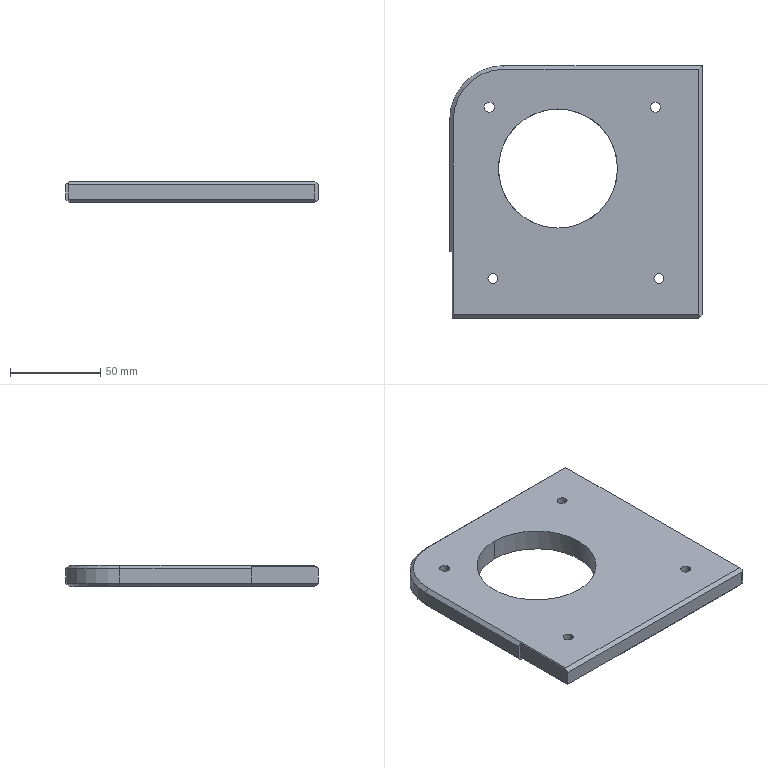Part | Creo | 1 solid | 43 faces | box 140 x 140 x 12 mm | volume 186778 mm3 | plane 22 | cylinder 19 | cone 2 | commonest cylinder face diameters 5.5 x8 9.5 x8 66 x2 60 x1
STEP:
#1=CARTESIAN_POINT('',(333.,-375.005,-1.));
#2=VERTEX_POINT('',#1);
#3=CARTESIAN_POINT('',(333.,-375.005,-9.));
#4=VERTEX_POINT('',#3);
#5=CARTESIAN_POINT('',(333.,-375.005,-1.));
#6=DIRECTION('',(0.,0.,-1.));
#7=VECTOR('',#6,8.);
#8=LINE('',#5,#7);
#9=EDGE_CURVE('',#2,#4,#8,.T.);
#10=ORIENTED_EDGE('',*,*,#9,.T.);
#11=CARTESIAN_POINT('',(196.5,-375.005,-9.));
#12=VERTEX_POINT('',#11);
#13=CARTESIAN_POINT('',(333.,-375.005,-9.));
#14=DIRECTION('',(-1.,0.,0.));
#15=VECTOR('',#14,136.5);
#16=LINE('',#13,#15);
#17=EDGE_CURVE('',#4,#12,#16,.T.);
#18=ORIENTED_EDGE('',*,*,#17,.T.);
#19=CARTESIAN_POINT('',(196.5,-375.005,-1.));
#20=VERTEX_POINT('',#19);
#21=CARTESIAN_POINT('',(196.5,-375.005,-1.));
#22=DIRECTION('',(0.,0.,-1.));
#23=VECTOR('',#22,8.);
#24=LINE('',#21,#23);
#25=EDGE_CURVE('',#20,#12,#24,.T.);
#26=ORIENTED_EDGE('',*,*,#25,.F.);
#27=CARTESIAN_POINT('',(196.5,-375.005,-1.));
#28=DIRECTION('',(1.,0.,0.));
#29=VECTOR('',#28,136.5);
#30=LINE('',#27,#29);
#31=EDGE_CURVE('',#20,#2,#30,.T.);
#32=ORIENTED_EDGE('',*,*,#31,.T.);
#33=EDGE_LOOP('',(#10,#18,#26,#32));
#34=FACE_OUTER_BOUND('',#33,.F.);
#35=CARTESIAN_POINT('',(-265.,-375.005,165.));
#36=DIRECTION('',(0.,-1.,0.));
#37=DIRECTION('',(0.,0.,-1.));
#38=AXIS2_PLACEMENT_3D('',#35,#36,#37);
#39=PLANE('',#38);
#40=ADVANCED_FACE('',(#34),#39,.T.);
#41=CARTESIAN_POINT('',(335.,-373.005,-9.));
#42=VERTEX_POINT('',#41);
#43=CARTESIAN_POINT('',(335.,-373.005,-1.));
#44=VERTEX_POINT('',#43);
#45=CARTESIAN_POINT('',(335.,-373.005,-9.));
#46=DIRECTION('',(0.,0.,1.));
#47=VECTOR('',#46,8.);
#48=LINE('',#45,#47);
#49=EDGE_CURVE('',#42,#44,#48,.T.);
#50=ORIENTED_EDGE('',*,*,#49,.F.);
#51=CARTESIAN_POINT('',(334.,-374.005,-10.));
#52=VERTEX_POINT('',#51);
#53=CARTESIAN_POINT('',(334.,-374.005,-10.));
#54=DIRECTION('',(0.5774,0.5774,0.5774));
#55=VECTOR('',#54,1.732);
#56=LINE('',#53,#55);
#57=EDGE_CURVE('',#52,#42,#56,.T.);
#58=ORIENTED_EDGE('',*,*,#57,.F.);
#59=CARTESIAN_POINT('',(333.,-375.005,-9.));
#60=DIRECTION('',(0.5774,0.5774,-0.5774));
#61=VECTOR('',#60,1.732);
#62=LINE('',#59,#61);
#63=EDGE_CURVE('',#4,#52,#62,.T.);
#64=ORIENTED_EDGE('',*,*,#63,.F.);
#65=ORIENTED_EDGE('',*,*,#9,.F.);
#66=CARTESIAN_POINT('',(334.,-374.005,0.));
#67=VERTEX_POINT('',#66);
#68=CARTESIAN_POINT('',(333.,-375.005,-1.));
#69=DIRECTION('',(0.5774,0.5774,0.5774));
#70=VECTOR('',#69,1.732);
#71=LINE('',#68,#70);
#72=EDGE_CURVE('',#2,#67,#71,.T.);
#73=ORIENTED_EDGE('',*,*,#72,.T.);
#74=CARTESIAN_POINT('',(334.,-374.005,0.));
#75=DIRECTION('',(0.5774,0.5774,-0.5774));
#76=VECTOR('',#75,1.732);
#77=LINE('',#74,#76);
#78=EDGE_CURVE('',#67,#44,#77,.T.);
#79=ORIENTED_EDGE('',*,*,#78,.T.);
#80=EDGE_LOOP('',(#50,#58,#64,#65,#73,#79));
#81=FACE_OUTER_BOUND('',#80,.F.);
#82=CARTESIAN_POINT('',(333.,-375.005,165.));
#83=DIRECTION('',(-0.7071,0.7071,0.));
#84=DIRECTION('',(0.,0.,1.));
#85=AXIS2_PLACEMENT_3D('',#82,#83,#84);
#86=PLANE('',#85);
#87=ADVANCED_FACE('',(#81),#86,.F.);
#88=CARTESIAN_POINT('',(335.,-235.005,-1.));
#89=VERTEX_POINT('',#88);
#90=CARTESIAN_POINT('',(335.,-235.005,-9.));
#91=VERTEX_POINT('',#90);
#92=CARTESIAN_POINT('',(335.,-235.005,-1.));
#93=DIRECTION('',(0.,0.,-1.));
#94=VECTOR('',#93,8.);
#95=LINE('',#92,#94);
#96=EDGE_CURVE('',#89,#91,#95,.T.);
#97=ORIENTED_EDGE('',*,*,#96,.T.);
#98=CARTESIAN_POINT('',(335.,-235.005,-9.));
#99=DIRECTION('',(0.,-1.,0.));
#100=VECTOR('',#99,138.);
#101=LINE('',#98,#100);
#102=EDGE_CURVE('',#91,#42,#101,.T.);
#103=ORIENTED_EDGE('',*,*,#102,.T.);
#104=ORIENTED_EDGE('',*,*,#49,.T.);
#105=CARTESIAN_POINT('',(335.,-373.005,-1.));
#106=DIRECTION('',(0.,1.,0.));
#107=VECTOR('',#106,138.);
#108=LINE('',#105,#107);
#109=EDGE_CURVE('',#44,#89,#108,.T.);
#110=ORIENTED_EDGE('',*,*,#109,.T.);
#111=EDGE_LOOP('',(#97,#103,#104,#110));
#112=FACE_OUTER_BOUND('',#111,.F.);
#113=CARTESIAN_POINT('',(335.,-50.005,5.));
#114=DIRECTION('',(1.,0.,0.));
#115=DIRECTION('',(0.,-1.,0.));
#116=AXIS2_PLACEMENT_3D('',#113,#114,#115);
#117=PLANE('',#116);
#118=ADVANCED_FACE('',(#112),#117,.T.);
#119=ORIENTED_EDGE('',*,*,#96,.F.);
#120=CARTESIAN_POINT('',(225.,-235.005,-1.));
#121=VERTEX_POINT('',#120);
#122=CARTESIAN_POINT('',(335.,-235.005,-1.));
#123=DIRECTION('',(-1.,0.,0.));
#124=VECTOR('',#123,110.);
#125=LINE('',#122,#124);
#126=EDGE_CURVE('',#89,#121,#125,.T.);
#127=ORIENTED_EDGE('',*,*,#126,.T.);
#128=CARTESIAN_POINT('',(225.,-235.005,-9.));
#129=VERTEX_POINT('',#128);
#130=CARTESIAN_POINT('',(225.,-235.005,-1.));
#131=DIRECTION('',(0.,0.,-1.));
#132=VECTOR('',#131,8.);
#133=LINE('',#130,#132);
#134=EDGE_CURVE('',#121,#129,#133,.T.);
#135=ORIENTED_EDGE('',*,*,#134,.T.);
#136=CARTESIAN_POINT('',(225.,-235.005,-9.));
#137=DIRECTION('',(1.,0.,0.));
#138=VECTOR('',#137,110.);
#139=LINE('',#136,#138);
#140=EDGE_CURVE('',#129,#91,#139,.T.);
#141=ORIENTED_EDGE('',*,*,#140,.T.);
#142=EDGE_LOOP('',(#119,#127,#135,#141));
#143=FACE_OUTER_BOUND('',#142,.F.);
#144=CARTESIAN_POINT('',(245.,-235.005,-10.));
#145=DIRECTION('',(0.,1.,0.));
#146=DIRECTION('',(0.,0.,1.));
#147=AXIS2_PLACEMENT_3D('',#144,#145,#146);
#148=PLANE('',#147);
#149=ADVANCED_FACE('',(#143),#148,.T.);
#150=CARTESIAN_POINT('',(225.,-237.005,1.));
#151=VERTEX_POINT('',#150);
#152=CARTESIAN_POINT('',(333.,-237.005,1.));
#153=VERTEX_POINT('',#152);
#154=CARTESIAN_POINT('',(225.,-237.005,1.));
#155=DIRECTION('',(1.,0.,0.));
#156=VECTOR('',#155,108.);
#157=LINE('',#154,#156);
#158=EDGE_CURVE('',#151,#153,#157,.T.);
#159=ORIENTED_EDGE('',*,*,#158,.F.);
#160=CARTESIAN_POINT('',(225.,-237.005,1.));
#161=DIRECTION('',(0.,0.7071,-0.7071));
#162=VECTOR('',#161,2.828);
#163=LINE('',#160,#162);
#164=EDGE_CURVE('',#151,#121,#163,.T.);
#165=ORIENTED_EDGE('',*,*,#164,.T.);
#166=ORIENTED_EDGE('',*,*,#126,.F.);
#167=CARTESIAN_POINT('',(335.,-235.005,-1.));
#168=DIRECTION('',(-0.5774,-0.5774,0.5774));
#169=VECTOR('',#168,3.464);
#170=LINE('',#167,#169);
#171=EDGE_CURVE('',#89,#153,#170,.T.);
#172=ORIENTED_EDGE('',*,*,#171,.T.);
#173=EDGE_LOOP('',(#159,#165,#166,#172));
#174=FACE_OUTER_BOUND('',#173,.F.);
#175=CARTESIAN_POINT('',(245.,-235.005,-1.));
#176=DIRECTION('',(0.,-0.7071,-0.7071));
#177=DIRECTION('',(1.,0.,0.));
#178=AXIS2_PLACEMENT_3D('',#175,#176,#177);
#179=PLANE('',#178);
#180=ADVANCED_FACE('',(#174),#179,.F.);
#181=CARTESIAN_POINT('',(333.,-373.005,1.));
#182=VERTEX_POINT('',#181);
#183=CARTESIAN_POINT('',(197.,-373.005,1.));
#184=VERTEX_POINT('',#183);
#185=CARTESIAN_POINT('',(333.,-373.005,1.));
#186=DIRECTION('',(-1.,0.,0.));
#187=VECTOR('',#186,136.);
#188=LINE('',#185,#187);
#189=EDGE_CURVE('',#182,#184,#188,.T.);
#190=ORIENTED_EDGE('',*,*,#189,.T.);
#191=CARTESIAN_POINT('',(197.,-265.005,1.));
#192=VERTEX_POINT('',#191);
#193=CARTESIAN_POINT('',(197.,-373.005,1.));
#194=DIRECTION('',(0.,1.,0.));
#195=VECTOR('',#194,108.);
#196=LINE('',#193,#195);
#197=EDGE_CURVE('',#184,#192,#196,.T.);
#198=ORIENTED_EDGE('',*,*,#197,.T.);
#199=CARTESIAN_POINT('',(225.,-265.005,1.));
#200=DIRECTION('',(0.,0.,1.));
#201=DIRECTION('',(0.,1.,0.));
#202=AXIS2_PLACEMENT_3D('',#199,#200,#201);
#203=CIRCLE('',#202,28.);
#204=EDGE_CURVE('',#151,#192,#203,.T.);
#205=ORIENTED_EDGE('',*,*,#204,.F.);
#206=ORIENTED_EDGE('',*,*,#158,.T.);
#207=CARTESIAN_POINT('',(333.,-237.005,1.));
#208=DIRECTION('',(0.,-1.,0.));
#209=VECTOR('',#208,136.);
#210=LINE('',#207,#209);
#211=EDGE_CURVE('',#153,#182,#210,.T.);
#212=ORIENTED_EDGE('',*,*,#211,.T.);
#213=EDGE_LOOP('',(#190,#198,#205,#206,#212));
#214=FACE_OUTER_BOUND('',#213,.F.);
#215=CARTESIAN_POINT('',(306.25,-258.009,1.));
#216=VERTEX_POINT('',#215);
#217=CARTESIAN_POINT('',(311.75,-258.009,1.));
#218=VERTEX_POINT('',#217);
#219=CARTESIAN_POINT('',(309.,-258.009,1.));
#220=DIRECTION('',(0.,0.,-1.));
#221=DIRECTION('',(-1.,0.,0.));
#222=AXIS2_PLACEMENT_3D('',#219,#220,#221);
#223=CIRCLE('',#222,2.75);
#224=EDGE_CURVE('',#216,#218,#223,.T.);
#225=ORIENTED_EDGE('',*,*,#224,.F.);
#226=CARTESIAN_POINT('',(309.,-258.009,1.));
#227=DIRECTION('',(0.,0.,-1.));
#228=DIRECTION('',(1.,0.,0.));
#229=AXIS2_PLACEMENT_3D('',#226,#227,#228);
#230=CIRCLE('',#229,2.75);
#231=EDGE_CURVE('',#218,#216,#230,.T.);
#232=ORIENTED_EDGE('',*,*,#231,.F.);
#233=EDGE_LOOP('',(#225,#232));
#234=FACE_BOUND('',#233,.F.);
#235=CARTESIAN_POINT('',(216.199,-353.009,1.));
#236=VERTEX_POINT('',#235);
#237=CARTESIAN_POINT('',(221.699,-353.009,1.));
#238=VERTEX_POINT('',#237);
#239=CARTESIAN_POINT('',(218.949,-353.009,1.));
#240=DIRECTION('',(0.,0.,-1.));
#241=DIRECTION('',(-1.,0.,0.));
#242=AXIS2_PLACEMENT_3D('',#239,#240,#241);
#243=CIRCLE('',#242,2.75);
#244=EDGE_CURVE('',#236,#238,#243,.T.);
#245=ORIENTED_EDGE('',*,*,#244,.F.);
#246=CARTESIAN_POINT('',(218.949,-353.009,1.));
#247=DIRECTION('',(0.,0.,-1.));
#248=DIRECTION('',(1.,0.,0.));
#249=AXIS2_PLACEMENT_3D('',#246,#247,#248);
#250=CIRCLE('',#249,2.75);
#251=EDGE_CURVE('',#238,#236,#250,.T.);
#252=ORIENTED_EDGE('',*,*,#251,.F.);
#253=EDGE_LOOP('',(#245,#252));
#254=FACE_BOUND('',#253,.F.);
#255=CARTESIAN_POINT('',(288.,-292.005,1.));
#256=VERTEX_POINT('',#255);
#257=CARTESIAN_POINT('',(255.,-325.005,1.));
#258=VERTEX_POINT('',#257);
#259=CARTESIAN_POINT('',(255.,-292.005,1.));
#260=DIRECTION('',(0.,0.,-1.));
#261=DIRECTION('',(1.,0.,0.));
#262=AXIS2_PLACEMENT_3D('',#259,#260,#261);
#263=CIRCLE('',#262,33.);
#264=EDGE_CURVE('',#256,#258,#263,.T.);
#265=ORIENTED_EDGE('',*,*,#264,.F.);
#266=CARTESIAN_POINT('',(255.,-259.005,1.));
#267=VERTEX_POINT('',#266);
#268=CARTESIAN_POINT('',(255.,-292.005,1.));
#269=DIRECTION('',(0.,0.,-1.));
#270=DIRECTION('',(0.,1.,0.));
#271=AXIS2_PLACEMENT_3D('',#268,#269,#270);
#272=CIRCLE('',#271,33.);
#273=EDGE_CURVE('',#267,#256,#272,.T.);
#274=ORIENTED_EDGE('',*,*,#273,.F.);
#275=CARTESIAN_POINT('',(255.,-292.005,1.));
#276=DIRECTION('',(0.,0.,-1.));
#277=DIRECTION('',(0.,-1.,0.));
#278=AXIS2_PLACEMENT_3D('',#275,#276,#277);
#279=CIRCLE('',#278,33.);
#280=EDGE_CURVE('',#258,#267,#279,.T.);
#281=ORIENTED_EDGE('',*,*,#280,.F.);
#282=EDGE_LOOP('',(#265,#274,#281));
#283=FACE_BOUND('',#282,.F.);
#284=CARTESIAN_POINT('',(214.25,-258.009,1.));
#285=VERTEX_POINT('',#284);
#286=CARTESIAN_POINT('',(219.75,-258.009,1.));
#287=VERTEX_POINT('',#286);
#288=CARTESIAN_POINT('',(217.,-258.009,1.));
#289=DIRECTION('',(0.,0.,-1.));
#290=DIRECTION('',(-1.,0.,0.));
#291=AXIS2_PLACEMENT_3D('',#288,#289,#290);
#292=CIRCLE('',#291,2.75);
#293=EDGE_CURVE('',#285,#287,#292,.T.);
#294=ORIENTED_EDGE('',*,*,#293,.F.);
#295=CARTESIAN_POINT('',(217.,-258.009,1.));
#296=DIRECTION('',(0.,0.,-1.));
#297=DIRECTION('',(1.,0.,0.));
#298=AXIS2_PLACEMENT_3D('',#295,#296,#297);
#299=CIRCLE('',#298,2.75);
#300=EDGE_CURVE('',#287,#285,#299,.T.);
#301=ORIENTED_EDGE('',*,*,#300,.F.);
#302=EDGE_LOOP('',(#294,#301));
#303=FACE_BOUND('',#302,.F.);
#304=CARTESIAN_POINT('',(308.199,-353.009,1.));
#305=VERTEX_POINT('',#304);
#306=CARTESIAN_POINT('',(313.699,-353.009,1.));
#307=VERTEX_POINT('',#306);
#308=CARTESIAN_POINT('',(310.949,-353.009,1.));
#309=DIRECTION('',(0.,0.,-1.));
#310=DIRECTION('',(-1.,0.,0.));
#311=AXIS2_PLACEMENT_3D('',#308,#309,#310);
#312=CIRCLE('',#311,2.75);
#313=EDGE_CURVE('',#305,#307,#312,.T.);
#314=ORIENTED_EDGE('',*,*,#313,.F.);
#315=CARTESIAN_POINT('',(310.949,-353.009,1.));
#316=DIRECTION('',(0.,0.,-1.));
#317=DIRECTION('',(1.,0.,0.));
#318=AXIS2_PLACEMENT_3D('',#315,#316,#317);
#319=CIRCLE('',#318,2.75);
#320=EDGE_CURVE('',#307,#305,#319,.T.);
#321=ORIENTED_EDGE('',*,*,#320,.F.);
#322=EDGE_LOOP('',(#314,#321));
#323=FACE_BOUND('',#322,.F.);
#324=CARTESIAN_POINT('',(245.,-302.505,1.));
#325=DIRECTION('',(0.,0.,1.));
#326=DIRECTION('',(1.,0.,0.));
#327=AXIS2_PLACEMENT_3D('',#324,#325,#326);
#328=PLANE('',#327);
#329=ADVANCED_FACE('',(#214,#234,#254,#283,#303,#323),#328,.T.);
#330=ORIENTED_EDGE('',*,*,#72,.F.);
#331=ORIENTED_EDGE('',*,*,#31,.F.);
#332=CARTESIAN_POINT('',(196.5,-373.505,0.5));
#333=VERTEX_POINT('',#332);
#334=CARTESIAN_POINT('',(196.5,-375.005,-1.));
#335=DIRECTION('',(0.,0.7071,0.7071));
#336=VECTOR('',#335,2.121);
#337=LINE('',#334,#336);
#338=EDGE_CURVE('',#20,#333,#337,.T.);
#339=ORIENTED_EDGE('',*,*,#338,.T.);
#340=CARTESIAN_POINT('',(197.,-373.005,1.));
#341=DIRECTION('',(-0.5774,-0.5774,-0.5774));
#342=VECTOR('',#341,0.866);
#343=LINE('',#340,#342);
#344=EDGE_CURVE('',#184,#333,#343,.T.);
#345=ORIENTED_EDGE('',*,*,#344,.F.);
#346=ORIENTED_EDGE('',*,*,#189,.F.);
#347=CARTESIAN_POINT('',(333.,-373.005,1.));
#348=DIRECTION('',(0.5774,-0.5774,-0.5774));
#349=VECTOR('',#348,1.732);
#350=LINE('',#347,#349);
#351=EDGE_CURVE('',#182,#67,#350,.T.);
#352=ORIENTED_EDGE('',*,*,#351,.T.);
#353=EDGE_LOOP('',(#330,#331,#339,#345,#346,#352));
#354=FACE_OUTER_BOUND('',#353,.F.);
#355=CARTESIAN_POINT('',(245.,-373.005,1.));
#356=DIRECTION('',(0.,0.7071,-0.7071));
#357=DIRECTION('',(1.,0.,0.));
#358=AXIS2_PLACEMENT_3D('',#355,#356,#357);
#359=PLANE('',#358);
#360=ADVANCED_FACE('',(#354),#359,.F.);
#361=ORIENTED_EDGE('',*,*,#25,.T.);
#362=CARTESIAN_POINT('',(196.5,-338.005,-9.));
#363=VERTEX_POINT('',#362);
#364=CARTESIAN_POINT('',(196.5,-375.005,-9.));
#365=DIRECTION('',(0.,1.,0.));
#366=VECTOR('',#365,37.);
#367=LINE('',#364,#366);
#368=EDGE_CURVE('',#12,#363,#367,.T.);
#369=ORIENTED_EDGE('',*,*,#368,.T.);
#370=CARTESIAN_POINT('',(196.5,-338.005,0.5));
#371=VERTEX_POINT('',#370);
#372=CARTESIAN_POINT('',(196.5,-338.005,-9.));
#373=DIRECTION('',(0.,0.,1.));
#374=VECTOR('',#373,9.5);
#375=LINE('',#372,#374);
#376=EDGE_CURVE('',#363,#371,#375,.T.);
#377=ORIENTED_EDGE('',*,*,#376,.T.);
#378=CARTESIAN_POINT('',(196.5,-338.005,0.5));
#379=DIRECTION('',(0.,-1.,0.));
#380=VECTOR('',#379,35.5);
#381=LINE('',#378,#380);
#382=EDGE_CURVE('',#371,#333,#381,.T.);
#383=ORIENTED_EDGE('',*,*,#382,.T.);
#384=ORIENTED_EDGE('',*,*,#338,.F.);
#385=EDGE_LOOP('',(#361,#369,#377,#383,#384));
#386=FACE_OUTER_BOUND('',#385,.F.);
#387=CARTESIAN_POINT('',(196.5,-394.005,-194.076));
#388=DIRECTION('',(1.,0.,0.));
#389=DIRECTION('',(0.,0.,1.));
#390=AXIS2_PLACEMENT_3D('',#387,#388,#389);
#391=PLANE('',#390);
#392=ADVANCED_FACE('',(#386),#391,.F.);
#393=CARTESIAN_POINT('',(198.5,-338.005,-11.));
#394=VERTEX_POINT('',#393);
#395=CARTESIAN_POINT('',(198.5,-338.005,-11.));
#396=DIRECTION('',(-0.7071,0.,0.7071));
#397=VECTOR('',#396,2.828);
#398=LINE('',#395,#397);
#399=EDGE_CURVE('',#394,#363,#398,.T.);
#400=ORIENTED_EDGE('',*,*,#399,.T.);
#401=ORIENTED_EDGE('',*,*,#368,.F.);
#402=CARTESIAN_POINT('',(198.5,-373.005,-11.));
#403=VERTEX_POINT('',#402);
#404=CARTESIAN_POINT('',(198.5,-373.005,-11.));
#405=DIRECTION('',(-0.5774,-0.5774,0.5774));
#406=VECTOR('',#405,3.464);
#407=LINE('',#404,#406);
#408=EDGE_CURVE('',#403,#12,#407,.T.);
#409=ORIENTED_EDGE('',*,*,#408,.F.);
#410=CARTESIAN_POINT('',(198.5,-338.005,-11.));
#411=DIRECTION('',(0.,-1.,0.));
#412=VECTOR('',#411,35.);
#413=LINE('',#410,#412);
#414=EDGE_CURVE('',#394,#403,#413,.T.);
#415=ORIENTED_EDGE('',*,*,#414,.F.);
#416=EDGE_LOOP('',(#400,#401,#409,#415));
#417=FACE_OUTER_BOUND('',#416,.F.);
#418=CARTESIAN_POINT('',(196.5,-394.005,-9.));
#419=DIRECTION('',(-0.7071,0.,-0.7071));
#420=DIRECTION('',(0.,1.,0.));
#421=AXIS2_PLACEMENT_3D('',#418,#419,#420);
#422=PLANE('',#421);
#423=ADVANCED_FACE('',(#417),#422,.T.);
#424=CARTESIAN_POINT('',(195.,-338.005,-9.));
#425=VERTEX_POINT('',#424);
#426=CARTESIAN_POINT('',(195.,-338.005,-1.));
#427=VERTEX_POINT('',#426);
#428=CARTESIAN_POINT('',(195.,-338.005,-9.));
#429=DIRECTION('',(0.,0.,1.));
#430=VECTOR('',#429,8.);
#431=LINE('',#428,#430);
#432=EDGE_CURVE('',#425,#427,#431,.T.);
#433=ORIENTED_EDGE('',*,*,#432,.T.);
#434=CARTESIAN_POINT('',(196.5,-338.005,0.5));
#435=DIRECTION('',(-0.7071,0.,-0.7071));
#436=VECTOR('',#435,2.121);
#437=LINE('',#434,#436);
#438=EDGE_CURVE('',#371,#427,#437,.T.);
#439=ORIENTED_EDGE('',*,*,#438,.F.);
#440=ORIENTED_EDGE('',*,*,#376,.F.);
#441=ORIENTED_EDGE('',*,*,#399,.F.);
#442=CARTESIAN_POINT('',(197.,-338.005,-11.));
#443=VERTEX_POINT('',#442);
#444=CARTESIAN_POINT('',(198.5,-338.005,-11.));
#445=DIRECTION('',(-1.,0.,0.));
#446=VECTOR('',#445,1.5);
#447=LINE('',#444,#446);
#448=EDGE_CURVE('',#394,#443,#447,.T.);
#449=ORIENTED_EDGE('',*,*,#448,.T.);
#450=CARTESIAN_POINT('',(195.,-338.005,-9.));
#451=DIRECTION('',(0.7071,0.,-0.7071));
#452=VECTOR('',#451,2.828);
#453=LINE('',#450,#452);
#454=EDGE_CURVE('',#425,#443,#453,.T.);
#455=ORIENTED_EDGE('',*,*,#454,.F.);
#456=EDGE_LOOP('',(#433,#439,#440,#441,#449,#455));
#457=FACE_OUTER_BOUND('',#456,.F.);
#458=CARTESIAN_POINT('',(175.,-338.005,-20.));
#459=DIRECTION('',(0.,-1.,0.));
#460=DIRECTION('',(1.,0.,0.));
#461=AXIS2_PLACEMENT_3D('',#458,#459,#460);
#462=PLANE('',#461);
#463=ADVANCED_FACE('',(#457),#462,.T.);
#464=CARTESIAN_POINT('',(195.,-265.005,-9.));
#465=VERTEX_POINT('',#464);
#466=CARTESIAN_POINT('',(195.,-265.005,-1.));
#467=VERTEX_POINT('',#466);
#468=CARTESIAN_POINT('',(195.,-265.005,-9.));
#469=DIRECTION('',(0.,0.,1.));
#470=VECTOR('',#469,8.);
#471=LINE('',#468,#470);
#472=EDGE_CURVE('',#465,#467,#471,.T.);
#473=ORIENTED_EDGE('',*,*,#472,.T.);
#474=CARTESIAN_POINT('',(195.,-265.005,-1.));
#475=DIRECTION('',(0.,-1.,0.));
#476=VECTOR('',#475,73.);
#477=LINE('',#474,#476);
#478=EDGE_CURVE('',#467,#427,#477,.T.);
#479=ORIENTED_EDGE('',*,*,#478,.T.);
#480=ORIENTED_EDGE('',*,*,#432,.F.);
#481=CARTESIAN_POINT('',(195.,-338.005,-9.));
#482=DIRECTION('',(0.,1.,0.));
#483=VECTOR('',#482,73.);
#484=LINE('',#481,#483);
#485=EDGE_CURVE('',#425,#465,#484,.T.);
#486=ORIENTED_EDGE('',*,*,#485,.T.);
#487=EDGE_LOOP('',(#473,#479,#480,#486));
#488=FACE_OUTER_BOUND('',#487,.F.);
#489=CARTESIAN_POINT('',(195.,-0.004699,1.));
#490=DIRECTION('',(1.,0.,0.));
#491=DIRECTION('',(0.,-1.,0.));
#492=AXIS2_PLACEMENT_3D('',#489,#490,#491);
#493=PLANE('',#492);
#494=ADVANCED_FACE('',(#488),#493,.F.);
#495=ORIENTED_EDGE('',*,*,#134,.F.);
#496=CARTESIAN_POINT('',(225.,-265.005,-1.));
#497=DIRECTION('',(0.,0.,1.));
#498=DIRECTION('',(0.,1.,0.));
#499=AXIS2_PLACEMENT_3D('',#496,#497,#498);
#500=CIRCLE('',#499,30.);
#501=EDGE_CURVE('',#121,#467,#500,.T.);
#502=ORIENTED_EDGE('',*,*,#501,.T.);
#503=ORIENTED_EDGE('',*,*,#472,.F.);
#504=CARTESIAN_POINT('',(225.,-265.005,-9.));
#505=DIRECTION('',(0.,0.,-1.));
#506=DIRECTION('',(-1.,0.,0.));
#507=AXIS2_PLACEMENT_3D('',#504,#505,#506);
#508=CIRCLE('',#507,30.);
#509=EDGE_CURVE('',#465,#129,#508,.T.);
#510=ORIENTED_EDGE('',*,*,#509,.T.);
#511=EDGE_LOOP('',(#495,#502,#503,#510));
#512=FACE_OUTER_BOUND('',#511,.F.);
#513=CARTESIAN_POINT('',(225.,-265.005,-10.));
#514=DIRECTION('',(0.,0.,-1.));
#515=DIRECTION('',(-1.,0.,0.));
#516=AXIS2_PLACEMENT_3D('',#513,#514,#515);
#517=CYLINDRICAL_SURFACE('',#516,30.);
#518=ADVANCED_FACE('',(#512),#517,.T.);
#519=ORIENTED_EDGE('',*,*,#164,.F.);
#520=ORIENTED_EDGE('',*,*,#204,.T.);
#521=CARTESIAN_POINT('',(195.,-265.005,-1.));
#522=DIRECTION('',(0.7071,0.,0.7071));
#523=VECTOR('',#522,2.828);
#524=LINE('',#521,#523);
#525=EDGE_CURVE('',#467,#192,#524,.T.);
#526=ORIENTED_EDGE('',*,*,#525,.F.);
#527=ORIENTED_EDGE('',*,*,#501,.F.);
#528=EDGE_LOOP('',(#519,#520,#526,#527));
#529=FACE_OUTER_BOUND('',#528,.F.);
#530=CARTESIAN_POINT('',(225.,-265.005,0.));
#531=DIRECTION('',(0.,0.,-1.));
#532=DIRECTION('',(-1.,0.,0.));
#533=AXIS2_PLACEMENT_3D('',#530,#531,#532);
#534=CONICAL_SURFACE('',#533,29.,45.);
#535=ADVANCED_FACE('',(#529),#534,.T.);
#536=ORIENTED_EDGE('',*,*,#382,.F.);
#537=ORIENTED_EDGE('',*,*,#438,.T.);
#538=ORIENTED_EDGE('',*,*,#478,.F.);
#539=ORIENTED_EDGE('',*,*,#525,.T.);
#540=ORIENTED_EDGE('',*,*,#197,.F.);
#541=ORIENTED_EDGE('',*,*,#344,.T.);
#542=EDGE_LOOP('',(#536,#537,#538,#539,#540,#541));
#543=FACE_OUTER_BOUND('',#542,.F.);
#544=CARTESIAN_POINT('',(195.,-0.004699,-1.));
#545=DIRECTION('',(-0.7071,0.,0.7071));
#546=DIRECTION('',(0.,-1.,0.));
#547=AXIS2_PLACEMENT_3D('',#544,#545,#546);
#548=PLANE('',#547);
#549=ADVANCED_FACE('',(#543),#548,.T.);
#550=CARTESIAN_POINT('',(197.,-265.005,-11.));
#551=VERTEX_POINT('',#550);
#552=CARTESIAN_POINT('',(197.,-265.005,-11.));
#553=DIRECTION('',(-0.7071,0.,0.7071));
#554=VECTOR('',#553,2.828);
#555=LINE('',#552,#554);
#556=EDGE_CURVE('',#551,#465,#555,.T.);
#557=ORIENTED_EDGE('',*,*,#556,.F.);
#558=CARTESIAN_POINT('',(225.,-237.005,-11.));
#559=VERTEX_POINT('',#558);
#560=CARTESIAN_POINT('',(225.,-265.005,-11.));
#561=DIRECTION('',(0.,0.,-1.));
#562=DIRECTION('',(-1.,0.,0.));
#563=AXIS2_PLACEMENT_3D('',#560,#561,#562);
#564=CIRCLE('',#563,28.);
#565=EDGE_CURVE('',#551,#559,#564,.T.);
#566=ORIENTED_EDGE('',*,*,#565,.T.);
#567=CARTESIAN_POINT('',(225.,-235.005,-9.));
#568=DIRECTION('',(0.,-0.7071,-0.7071));
#569=VECTOR('',#568,2.828);
#570=LINE('',#567,#569);
#571=EDGE_CURVE('',#129,#559,#570,.T.);
#572=ORIENTED_EDGE('',*,*,#571,.F.);
#573=ORIENTED_EDGE('',*,*,#509,.F.);
#574=EDGE_LOOP('',(#557,#566,#572,#573));
#575=FACE_OUTER_BOUND('',#574,.F.);
#576=CARTESIAN_POINT('',(225.,-265.005,-10.));
#577=DIRECTION('',(0.,0.,1.));
#578=DIRECTION('',(1.,0.,0.));
#579=AXIS2_PLACEMENT_3D('',#576,#577,#578);
#580=CONICAL_SURFACE('',#579,29.,45.);
#581=ADVANCED_FACE('',(#575),#580,.T.);
#582=ORIENTED_EDGE('',*,*,#454,.T.);
#583=CARTESIAN_POINT('',(197.,-265.005,-11.));
#584=DIRECTION('',(0.,-1.,0.));
#585=VECTOR('',#584,73.);
#586=LINE('',#583,#585);
#587=EDGE_CURVE('',#551,#443,#586,.T.);
#588=ORIENTED_EDGE('',*,*,#587,.F.);
#589=ORIENTED_EDGE('',*,*,#556,.T.);
#590=ORIENTED_EDGE('',*,*,#485,.F.);
#591=EDGE_LOOP('',(#582,#588,#589,#590));
#592=FACE_OUTER_BOUND('',#591,.F.);
#593=CARTESIAN_POINT('',(195.,-0.004699,-9.));
#594=DIRECTION('',(-0.7071,0.,-0.7071));
#595=DIRECTION('',(0.,1.,0.));
#596=AXIS2_PLACEMENT_3D('',#593,#594,#595);
#597=PLANE('',#596);
#598=ADVANCED_FACE('',(#592),#597,.T.);
#599=ORIENTED_EDGE('',*,*,#565,.F.);
#600=ORIENTED_EDGE('',*,*,#587,.T.);
#601=ORIENTED_EDGE('',*,*,#448,.F.);
#602=ORIENTED_EDGE('',*,*,#414,.T.);
#603=CARTESIAN_POINT('',(333.,-373.005,-11.));
#604=VERTEX_POINT('',#603);
#605=CARTESIAN_POINT('',(198.5,-373.005,-11.));
#606=DIRECTION('',(1.,0.,0.));
#607=VECTOR('',#606,134.5);
#608=LINE('',#605,#607);
#609=EDGE_CURVE('',#403,#604,#608,.T.);
#610=ORIENTED_EDGE('',*,*,#609,.T.);
#611=CARTESIAN_POINT('',(333.,-237.005,-11.));
#612=VERTEX_POINT('',#611);
#613=CARTESIAN_POINT('',(333.,-373.005,-11.));
#614=DIRECTION('',(0.,1.,0.));
#615=VECTOR('',#614,136.);
#616=LINE('',#613,#615);
#617=EDGE_CURVE('',#604,#612,#616,.T.);
#618=ORIENTED_EDGE('',*,*,#617,.T.);
#619=CARTESIAN_POINT('',(333.,-237.005,-11.));
#620=DIRECTION('',(-1.,0.,0.));
#621=VECTOR('',#620,108.);
#622=LINE('',#619,#621);
#623=EDGE_CURVE('',#612,#559,#622,.T.);
#624=ORIENTED_EDGE('',*,*,#623,.T.);
#625=EDGE_LOOP('',(#599,#600,#601,#602,#610,#618,#624));
#626=FACE_OUTER_BOUND('',#625,.F.);
#627=CARTESIAN_POINT('',(214.199,-353.009,-11.));
#628=VERTEX_POINT('',#627);
#629=CARTESIAN_POINT('',(223.699,-353.009,-11.));
#630=VERTEX_POINT('',#629);
#631=CARTESIAN_POINT('',(218.949,-353.009,-11.));
#632=DIRECTION('',(0.,0.,1.));
#633=DIRECTION('',(-1.,0.,0.));
#634=AXIS2_PLACEMENT_3D('',#631,#632,#633);
#635=CIRCLE('',#634,4.75);
#636=EDGE_CURVE('',#628,#630,#635,.T.);
#637=ORIENTED_EDGE('',*,*,#636,.F.);
#638=CARTESIAN_POINT('',(218.949,-353.009,-11.));
#639=DIRECTION('',(0.,0.,1.));
#640=DIRECTION('',(1.,0.,0.));
#641=AXIS2_PLACEMENT_3D('',#638,#639,#640);
#642=CIRCLE('',#641,4.75);
#643=EDGE_CURVE('',#630,#628,#642,.T.);
#644=ORIENTED_EDGE('',*,*,#643,.F.);
#645=EDGE_LOOP('',(#637,#644));
#646=FACE_BOUND('',#645,.F.);
#647=CARTESIAN_POINT('',(306.199,-353.009,-11.));
#648=VERTEX_POINT('',#647);
#649=CARTESIAN_POINT('',(315.699,-353.009,-11.));
#650=VERTEX_POINT('',#649);
#651=CARTESIAN_POINT('',(310.949,-353.009,-11.));
#652=DIRECTION('',(0.,0.,1.));
#653=DIRECTION('',(-1.,0.,0.));
#654=AXIS2_PLACEMENT_3D('',#651,#652,#653);
#655=CIRCLE('',#654,4.75);
#656=EDGE_CURVE('',#648,#650,#655,.T.);
#657=ORIENTED_EDGE('',*,*,#656,.F.);
#658=CARTESIAN_POINT('',(310.949,-353.009,-11.));
#659=DIRECTION('',(0.,0.,1.));
#660=DIRECTION('',(1.,0.,0.));
#661=AXIS2_PLACEMENT_3D('',#658,#659,#660);
#662=CIRCLE('',#661,4.75);
#663=EDGE_CURVE('',#650,#648,#662,.T.);
#664=ORIENTED_EDGE('',*,*,#663,.F.);
#665=EDGE_LOOP('',(#657,#664));
#666=FACE_BOUND('',#665,.F.);
#667=CARTESIAN_POINT('',(304.25,-258.009,-11.));
#668=VERTEX_POINT('',#667);
#669=CARTESIAN_POINT('',(313.75,-258.009,-11.));
#670=VERTEX_POINT('',#669);
#671=CARTESIAN_POINT('',(309.,-258.009,-11.));
#672=DIRECTION('',(0.,0.,1.));
#673=DIRECTION('',(-1.,0.,0.));
#674=AXIS2_PLACEMENT_3D('',#671,#672,#673);
#675=CIRCLE('',#674,4.75);
#676=EDGE_CURVE('',#668,#670,#675,.T.);
#677=ORIENTED_EDGE('',*,*,#676,.F.);
#678=CARTESIAN_POINT('',(309.,-258.009,-11.));
#679=DIRECTION('',(0.,0.,1.));
#680=DIRECTION('',(1.,0.,0.));
#681=AXIS2_PLACEMENT_3D('',#678,#679,#680);
#682=CIRCLE('',#681,4.75);
#683=EDGE_CURVE('',#670,#668,#682,.T.);
#684=ORIENTED_EDGE('',*,*,#683,.F.);
#685=EDGE_LOOP('',(#677,#684));
#686=FACE_BOUND('',#685,.F.);
#687=CARTESIAN_POINT('',(212.25,-258.009,-11.));
#688=VERTEX_POINT('',#687);
#689=CARTESIAN_POINT('',(221.75,-258.009,-11.));
#690=VERTEX_POINT('',#689);
#691=CARTESIAN_POINT('',(217.,-258.009,-11.));
#692=DIRECTION('',(0.,0.,1.));
#693=DIRECTION('',(-1.,0.,0.));
#694=AXIS2_PLACEMENT_3D('',#691,#692,#693);
#695=CIRCLE('',#694,4.75);
#696=EDGE_CURVE('',#688,#690,#695,.T.);
#697=ORIENTED_EDGE('',*,*,#696,.F.);
#698=CARTESIAN_POINT('',(217.,-258.009,-11.));
#699=DIRECTION('',(0.,0.,1.));
#700=DIRECTION('',(1.,0.,0.));
#701=AXIS2_PLACEMENT_3D('',#698,#699,#700);
#702=CIRCLE('',#701,4.75);
#703=EDGE_CURVE('',#690,#688,#702,.T.);
#704=ORIENTED_EDGE('',*,*,#703,.F.);
#705=EDGE_LOOP('',(#697,#704));
#706=FACE_BOUND('',#705,.F.);
#707=CARTESIAN_POINT('',(222.,-292.005,-11.));
#708=VERTEX_POINT('',#707);
#709=CARTESIAN_POINT('',(255.,-325.005,-11.));
#710=VERTEX_POINT('',#709);
#711=CARTESIAN_POINT('',(255.,-292.005,-11.));
#712=DIRECTION('',(0.,0.,1.));
#713=DIRECTION('',(-1.,0.,0.));
#714=AXIS2_PLACEMENT_3D('',#711,#712,#713);
#715=CIRCLE('',#714,33.);
#716=EDGE_CURVE('',#708,#710,#715,.T.);
#717=ORIENTED_EDGE('',*,*,#716,.F.);
#718=CARTESIAN_POINT('',(255.,-259.005,-11.));
#719=VERTEX_POINT('',#718);
#720=CARTESIAN_POINT('',(255.,-292.005,-11.));
#721=DIRECTION('',(0.,0.,1.));
#722=DIRECTION('',(0.,1.,0.));
#723=AXIS2_PLACEMENT_3D('',#720,#721,#722);
#724=CIRCLE('',#723,33.);
#725=EDGE_CURVE('',#719,#708,#724,.T.);
#726=ORIENTED_EDGE('',*,*,#725,.F.);
#727=CARTESIAN_POINT('',(255.,-292.005,-11.));
#728=DIRECTION('',(0.,0.,1.));
#729=DIRECTION('',(0.,-1.,0.));
#730=AXIS2_PLACEMENT_3D('',#727,#728,#729);
#731=CIRCLE('',#730,33.);
#732=EDGE_CURVE('',#710,#719,#731,.T.);
#733=ORIENTED_EDGE('',*,*,#732,.F.);
#734=EDGE_LOOP('',(#717,#726,#733));
#735=FACE_BOUND('',#734,.F.);
#736=CARTESIAN_POINT('',(245.,-302.505,-11.));
#737=DIRECTION('',(0.,0.,-1.));
#738=DIRECTION('',(-1.,0.,0.));
#739=AXIS2_PLACEMENT_3D('',#736,#737,#738);
#740=PLANE('',#739);
#741=ADVANCED_FACE('',(#626,#646,#666,#686,#706,#735),#740,.T.);
#742=CARTESIAN_POINT('',(333.,-373.005,-11.));
#743=DIRECTION('',(0.5774,-0.5774,0.5774));
#744=VECTOR('',#743,1.732);
#745=LINE('',#742,#744);
#746=EDGE_CURVE('',#604,#52,#745,.T.);
#747=ORIENTED_EDGE('',*,*,#746,.F.);
#748=ORIENTED_EDGE('',*,*,#609,.F.);
#749=ORIENTED_EDGE('',*,*,#408,.T.);
#750=ORIENTED_EDGE('',*,*,#17,.F.);
#751=ORIENTED_EDGE('',*,*,#63,.T.);
#752=EDGE_LOOP('',(#747,#748,#749,#750,#751));
#753=FACE_OUTER_BOUND('',#752,.F.);
#754=CARTESIAN_POINT('',(-265.,-375.005,-9.));
#755=DIRECTION('',(0.,0.7071,0.7071));
#756=DIRECTION('',(1.,0.,0.));
#757=AXIS2_PLACEMENT_3D('',#754,#755,#756);
#758=PLANE('',#757);
#759=ADVANCED_FACE('',(#753),#758,.F.);
#760=ORIENTED_EDGE('',*,*,#617,.F.);
#761=ORIENTED_EDGE('',*,*,#746,.T.);
#762=ORIENTED_EDGE('',*,*,#57,.T.);
#763=ORIENTED_EDGE('',*,*,#102,.F.);
#764=CARTESIAN_POINT('',(335.,-235.005,-9.));
#765=DIRECTION('',(-0.5774,-0.5774,-0.5774));
#766=VECTOR('',#765,3.464);
#767=LINE('',#764,#766);
#768=EDGE_CURVE('',#91,#612,#767,.T.);
#769=ORIENTED_EDGE('',*,*,#768,.T.);
#770=EDGE_LOOP('',(#760,#761,#762,#763,#769));
#771=FACE_OUTER_BOUND('',#770,.F.);
#772=CARTESIAN_POINT('',(335.,-50.005,-9.));
#773=DIRECTION('',(-0.7071,0.,0.7071));
#774=DIRECTION('',(0.,1.,0.));
#775=AXIS2_PLACEMENT_3D('',#772,#773,#774);
#776=PLANE('',#775);
#777=ADVANCED_FACE('',(#771),#776,.F.);
#778=ORIENTED_EDGE('',*,*,#768,.F.);
#779=ORIENTED_EDGE('',*,*,#140,.F.);
#780=ORIENTED_EDGE('',*,*,#571,.T.);
#781=ORIENTED_EDGE('',*,*,#623,.F.);
#782=EDGE_LOOP('',(#778,#779,#780,#781));
#783=FACE_OUTER_BOUND('',#782,.F.);
#784=CARTESIAN_POINT('',(245.,-235.005,-9.));
#785=DIRECTION('',(0.,-0.7071,0.7071));
#786=DIRECTION('',(-1.,0.,0.));
#787=AXIS2_PLACEMENT_3D('',#784,#785,#786);
#788=PLANE('',#787);
#789=ADVANCED_FACE('',(#783),#788,.F.);
#790=ORIENTED_EDGE('',*,*,#636,.T.);
#791=CARTESIAN_POINT('',(223.699,-353.009,-5.));
#792=VERTEX_POINT('',#791);
#793=CARTESIAN_POINT('',(223.699,-353.009,-5.));
#794=DIRECTION('',(0.,0.,-1.));
#795=VECTOR('',#794,6.);
#796=LINE('',#793,#795);
#797=EDGE_CURVE('',#792,#630,#796,.T.);
#798=ORIENTED_EDGE('',*,*,#797,.F.);
#799=CARTESIAN_POINT('',(214.199,-353.009,-5.));
#800=VERTEX_POINT('',#799);
#801=CARTESIAN_POINT('',(218.949,-353.009,-5.));
#802=DIRECTION('',(0.,0.,-1.));
#803=DIRECTION('',(1.,0.,0.));
#804=AXIS2_PLACEMENT_3D('',#801,#802,#803);
#805=CIRCLE('',#804,4.75);
#806=EDGE_CURVE('',#792,#800,#805,.T.);
#807=ORIENTED_EDGE('',*,*,#806,.T.);
#808=CARTESIAN_POINT('',(214.199,-353.009,-5.));
#809=DIRECTION('',(0.,0.,-1.));
#810=VECTOR('',#809,6.);
#811=LINE('',#808,#810);
#812=EDGE_CURVE('',#800,#628,#811,.T.);
#813=ORIENTED_EDGE('',*,*,#812,.T.);
#814=EDGE_LOOP('',(#790,#798,#807,#813));
#815=FACE_OUTER_BOUND('',#814,.F.);
#816=CARTESIAN_POINT('',(218.949,-353.009,-11.));
#817=DIRECTION('',(0.,0.,-1.));
#818=DIRECTION('',(-1.,0.,0.));
#819=AXIS2_PLACEMENT_3D('',#816,#817,#818);
#820=CYLINDRICAL_SURFACE('',#819,4.75);
#821=ADVANCED_FACE('',(#815),#820,.F.);
#822=ORIENTED_EDGE('',*,*,#643,.T.);
#823=ORIENTED_EDGE('',*,*,#812,.F.);
#824=CARTESIAN_POINT('',(218.949,-353.009,-5.));
#825=DIRECTION('',(0.,0.,-1.));
#826=DIRECTION('',(-1.,0.,0.));
#827=AXIS2_PLACEMENT_3D('',#824,#825,#826);
#828=CIRCLE('',#827,4.75);
#829=EDGE_CURVE('',#800,#792,#828,.T.);
#830=ORIENTED_EDGE('',*,*,#829,.T.);
#831=ORIENTED_EDGE('',*,*,#797,.T.);
#832=EDGE_LOOP('',(#822,#823,#830,#831));
#833=FACE_OUTER_BOUND('',#832,.F.);
#834=CARTESIAN_POINT('',(218.949,-353.009,-11.));
#835=DIRECTION('',(0.,0.,-1.));
#836=DIRECTION('',(-1.,0.,0.));
#837=AXIS2_PLACEMENT_3D('',#834,#835,#836);
#838=CYLINDRICAL_SURFACE('',#837,4.75);
#839=ADVANCED_FACE('',(#833),#838,.F.);
#840=ORIENTED_EDGE('',*,*,#829,.F.);
#841=ORIENTED_EDGE('',*,*,#806,.F.);
#842=EDGE_LOOP('',(#840,#841));
#843=FACE_OUTER_BOUND('',#842,.F.);
#844=CARTESIAN_POINT('',(216.199,-353.009,-5.));
#845=VERTEX_POINT('',#844);
#846=CARTESIAN_POINT('',(221.699,-353.009,-5.));
#847=VERTEX_POINT('',#846);
#848=CARTESIAN_POINT('',(218.949,-353.009,-5.));
#849=DIRECTION('',(0.,0.,1.));
#850=DIRECTION('',(-1.,0.,0.));
#851=AXIS2_PLACEMENT_3D('',#848,#849,#850);
#852=CIRCLE('',#851,2.75);
#853=EDGE_CURVE('',#845,#847,#852,.T.);
#854=ORIENTED_EDGE('',*,*,#853,.F.);
#855=CARTESIAN_POINT('',(218.949,-353.009,-5.));
#856=DIRECTION('',(0.,0.,1.));
#857=DIRECTION('',(1.,0.,0.));
#858=AXIS2_PLACEMENT_3D('',#855,#856,#857);
#859=CIRCLE('',#858,2.75);
#860=EDGE_CURVE('',#847,#845,#859,.T.);
#861=ORIENTED_EDGE('',*,*,#860,.F.);
#862=EDGE_LOOP('',(#854,#861));
#863=FACE_BOUND('',#862,.F.);
#864=CARTESIAN_POINT('',(218.949,-348.259,-5.));
#865=DIRECTION('',(0.,0.,1.));
#866=DIRECTION('',(1.,0.,0.));
#867=AXIS2_PLACEMENT_3D('',#864,#865,#866);
#868=PLANE('',#867);
#869=ADVANCED_FACE('',(#843,#863),#868,.F.);
#870=ORIENTED_EDGE('',*,*,#251,.T.);
#871=CARTESIAN_POINT('',(216.199,-353.009,1.));
#872=DIRECTION('',(0.,0.,-1.));
#873=VECTOR('',#872,6.);
#874=LINE('',#871,#873);
#875=EDGE_CURVE('',#236,#845,#874,.T.);
#876=ORIENTED_EDGE('',*,*,#875,.T.);
#877=ORIENTED_EDGE('',*,*,#853,.T.);
#878=CARTESIAN_POINT('',(221.699,-353.009,1.));
#879=DIRECTION('',(0.,0.,-1.));
#880=VECTOR('',#879,6.);
#881=LINE('',#878,#880);
#882=EDGE_CURVE('',#238,#847,#881,.T.);
#883=ORIENTED_EDGE('',*,*,#882,.F.);
#884=EDGE_LOOP('',(#870,#876,#877,#883));
#885=FACE_OUTER_BOUND('',#884,.F.);
#886=CARTESIAN_POINT('',(218.949,-353.009,-11.));
#887=DIRECTION('',(0.,0.,-1.));
#888=DIRECTION('',(-1.,0.,0.));
#889=AXIS2_PLACEMENT_3D('',#886,#887,#888);
#890=CYLINDRICAL_SURFACE('',#889,2.75);
#891=ADVANCED_FACE('',(#885),#890,.F.);
#892=ORIENTED_EDGE('',*,*,#244,.T.);
#893=ORIENTED_EDGE('',*,*,#882,.T.);
#894=ORIENTED_EDGE('',*,*,#860,.T.);
#895=ORIENTED_EDGE('',*,*,#875,.F.);
#896=EDGE_LOOP('',(#892,#893,#894,#895));
#897=FACE_OUTER_BOUND('',#896,.F.);
#898=CARTESIAN_POINT('',(218.949,-353.009,-11.));
#899=DIRECTION('',(0.,0.,-1.));
#900=DIRECTION('',(-1.,0.,0.));
#901=AXIS2_PLACEMENT_3D('',#898,#899,#900);
#902=CYLINDRICAL_SURFACE('',#901,2.75);
#903=ADVANCED_FACE('',(#897),#902,.F.);
#904=CARTESIAN_POINT('',(315.699,-353.009,-5.));
#905=VERTEX_POINT('',#904);
#906=CARTESIAN_POINT('',(306.199,-353.009,-5.));
#907=VERTEX_POINT('',#906);
#908=CARTESIAN_POINT('',(310.949,-353.009,-5.));
#909=DIRECTION('',(0.,0.,-1.));
#910=DIRECTION('',(1.,0.,0.));
#911=AXIS2_PLACEMENT_3D('',#908,#909,#910);
#912=CIRCLE('',#911,4.75);
#913=EDGE_CURVE('',#905,#907,#912,.T.);
#914=ORIENTED_EDGE('',*,*,#913,.T.);
#915=CARTESIAN_POINT('',(306.199,-353.009,-5.));
#916=DIRECTION('',(0.,0.,-1.));
#917=VECTOR('',#916,6.);
#918=LINE('',#915,#917);
#919=EDGE_CURVE('',#907,#648,#918,.T.);
#920=ORIENTED_EDGE('',*,*,#919,.T.);
#921=ORIENTED_EDGE('',*,*,#656,.T.);
#922=CARTESIAN_POINT('',(315.699,-353.009,-5.));
#923=DIRECTION('',(0.,0.,-1.));
#924=VECTOR('',#923,6.);
#925=LINE('',#922,#924);
#926=EDGE_CURVE('',#905,#650,#925,.T.);
#927=ORIENTED_EDGE('',*,*,#926,.F.);
#928=EDGE_LOOP('',(#914,#920,#921,#927));
#929=FACE_OUTER_BOUND('',#928,.F.);
#930=CARTESIAN_POINT('',(310.949,-353.009,-11.));
#931=DIRECTION('',(0.,0.,-1.));
#932=DIRECTION('',(-1.,0.,0.));
#933=AXIS2_PLACEMENT_3D('',#930,#931,#932);
#934=CYLINDRICAL_SURFACE('',#933,4.75);
#935=ADVANCED_FACE('',(#929),#934,.F.);
#936=CARTESIAN_POINT('',(310.949,-353.009,-5.));
#937=DIRECTION('',(0.,0.,-1.));
#938=DIRECTION('',(-1.,0.,0.));
#939=AXIS2_PLACEMENT_3D('',#936,#937,#938);
#940=CIRCLE('',#939,4.75);
#941=EDGE_CURVE('',#907,#905,#940,.T.);
#942=ORIENTED_EDGE('',*,*,#941,.F.);
#943=ORIENTED_EDGE('',*,*,#913,.F.);
#944=EDGE_LOOP('',(#942,#943));
#945=FACE_OUTER_BOUND('',#944,.F.);
#946=CARTESIAN_POINT('',(308.199,-353.009,-5.));
#947=VERTEX_POINT('',#946);
#948=CARTESIAN_POINT('',(313.699,-353.009,-5.));
#949=VERTEX_POINT('',#948);
#950=CARTESIAN_POINT('',(310.949,-353.009,-5.));
#951=DIRECTION('',(0.,0.,1.));
#952=DIRECTION('',(-1.,0.,0.));
#953=AXIS2_PLACEMENT_3D('',#950,#951,#952);
#954=CIRCLE('',#953,2.75);
#955=EDGE_CURVE('',#947,#949,#954,.T.);
#956=ORIENTED_EDGE('',*,*,#955,.F.);
#957=CARTESIAN_POINT('',(310.949,-353.009,-5.));
#958=DIRECTION('',(0.,0.,1.));
#959=DIRECTION('',(1.,0.,0.));
#960=AXIS2_PLACEMENT_3D('',#957,#958,#959);
#961=CIRCLE('',#960,2.75);
#962=EDGE_CURVE('',#949,#947,#961,.T.);
#963=ORIENTED_EDGE('',*,*,#962,.F.);
#964=EDGE_LOOP('',(#956,#963));
#965=FACE_BOUND('',#964,.F.);
#966=CARTESIAN_POINT('',(310.949,-348.259,-5.));
#967=DIRECTION('',(0.,0.,1.));
#968=DIRECTION('',(1.,0.,0.));
#969=AXIS2_PLACEMENT_3D('',#966,#967,#968);
#970=PLANE('',#969);
#971=ADVANCED_FACE('',(#945,#965),#970,.F.);
#972=ORIENTED_EDGE('',*,*,#320,.T.);
#973=CARTESIAN_POINT('',(308.199,-353.009,1.));
#974=DIRECTION('',(0.,0.,-1.));
#975=VECTOR('',#974,6.);
#976=LINE('',#973,#975);
#977=EDGE_CURVE('',#305,#947,#976,.T.);
#978=ORIENTED_EDGE('',*,*,#977,.T.);
#979=ORIENTED_EDGE('',*,*,#955,.T.);
#980=CARTESIAN_POINT('',(313.699,-353.009,1.));
#981=DIRECTION('',(0.,0.,-1.));
#982=VECTOR('',#981,6.);
#983=LINE('',#980,#982);
#984=EDGE_CURVE('',#307,#949,#983,.T.);
#985=ORIENTED_EDGE('',*,*,#984,.F.);
#986=EDGE_LOOP('',(#972,#978,#979,#985));
#987=FACE_OUTER_BOUND('',#986,.F.);
#988=CARTESIAN_POINT('',(310.949,-353.009,-11.));
#989=DIRECTION('',(0.,0.,-1.));
#990=DIRECTION('',(-1.,0.,0.));
#991=AXIS2_PLACEMENT_3D('',#988,#989,#990);
#992=CYLINDRICAL_SURFACE('',#991,2.75);
#993=ADVANCED_FACE('',(#987),#992,.F.);
#994=ORIENTED_EDGE('',*,*,#313,.T.);
#995=ORIENTED_EDGE('',*,*,#984,.T.);
#996=ORIENTED_EDGE('',*,*,#962,.T.);
#997=ORIENTED_EDGE('',*,*,#977,.F.);
#998=EDGE_LOOP('',(#994,#995,#996,#997));
#999=FACE_OUTER_BOUND('',#998,.F.);
#1000=CARTESIAN_POINT('',(310.949,-353.009,-11.));
#1001=DIRECTION('',(0.,0.,-1.));
#1002=DIRECTION('',(-1.,0.,0.));
#1003=AXIS2_PLACEMENT_3D('',#1000,#1001,#1002);
#1004=CYLINDRICAL_SURFACE('',#1003,2.75);
#1005=ADVANCED_FACE('',(#999),#1004,.F.);
#1006=ORIENTED_EDGE('',*,*,#941,.T.);
#1007=ORIENTED_EDGE('',*,*,#926,.T.);
#1008=ORIENTED_EDGE('',*,*,#663,.T.);
#1009=ORIENTED_EDGE('',*,*,#919,.F.);
#1010=EDGE_LOOP('',(#1006,#1007,#1008,#1009));
#1011=FACE_OUTER_BOUND('',#1010,.F.);
#1012=CARTESIAN_POINT('',(310.949,-353.009,-11.));
#1013=DIRECTION('',(0.,0.,-1.));
#1014=DIRECTION('',(-1.,0.,0.));
#1015=AXIS2_PLACEMENT_3D('',#1012,#1013,#1014);
#1016=CYLINDRICAL_SURFACE('',#1015,4.75);
#1017=ADVANCED_FACE('',(#1011),#1016,.F.);
#1018=CARTESIAN_POINT('',(313.75,-258.009,-5.));
#1019=VERTEX_POINT('',#1018);
#1020=CARTESIAN_POINT('',(304.25,-258.009,-5.));
#1021=VERTEX_POINT('',#1020);
#1022=CARTESIAN_POINT('',(309.,-258.009,-5.));
#1023=DIRECTION('',(0.,0.,-1.));
#1024=DIRECTION('',(1.,0.,0.));
#1025=AXIS2_PLACEMENT_3D('',#1022,#1023,#1024);
#1026=CIRCLE('',#1025,4.75);
#1027=EDGE_CURVE('',#1019,#1021,#1026,.T.);
#1028=ORIENTED_EDGE('',*,*,#1027,.T.);
#1029=CARTESIAN_POINT('',(304.25,-258.009,-5.));
#1030=DIRECTION('',(0.,0.,-1.));
#1031=VECTOR('',#1030,6.);
#1032=LINE('',#1029,#1031);
#1033=EDGE_CURVE('',#1021,#668,#1032,.T.);
#1034=ORIENTED_EDGE('',*,*,#1033,.T.);
#1035=ORIENTED_EDGE('',*,*,#676,.T.);
#1036=CARTESIAN_POINT('',(313.75,-258.009,-5.));
#1037=DIRECTION('',(0.,0.,-1.));
#1038=VECTOR('',#1037,6.);
#1039=LINE('',#1036,#1038);
#1040=EDGE_CURVE('',#1019,#670,#1039,.T.);
#1041=ORIENTED_EDGE('',*,*,#1040,.F.);
#1042=EDGE_LOOP('',(#1028,#1034,#1035,#1041));
#1043=FACE_OUTER_BOUND('',#1042,.F.);
#1044=CARTESIAN_POINT('',(309.,-258.009,-11.));
#1045=DIRECTION('',(0.,0.,-1.));
#1046=DIRECTION('',(-1.,0.,0.));
#1047=AXIS2_PLACEMENT_3D('',#1044,#1045,#1046);
#1048=CYLINDRICAL_SURFACE('',#1047,4.75);
#1049=ADVANCED_FACE('',(#1043),#1048,.F.);
#1050=CARTESIAN_POINT('',(309.,-258.009,-5.));
#1051=DIRECTION('',(0.,0.,-1.));
#1052=DIRECTION('',(-1.,0.,0.));
#1053=AXIS2_PLACEMENT_3D('',#1050,#1051,#1052);
#1054=CIRCLE('',#1053,4.75);
#1055=EDGE_CURVE('',#1021,#1019,#1054,.T.);
#1056=ORIENTED_EDGE('',*,*,#1055,.F.);
#1057=ORIENTED_EDGE('',*,*,#1027,.F.);
#1058=EDGE_LOOP('',(#1056,#1057));
#1059=FACE_OUTER_BOUND('',#1058,.F.);
#1060=CARTESIAN_POINT('',(306.25,-258.009,-5.));
#1061=VERTEX_POINT('',#1060);
#1062=CARTESIAN_POINT('',(311.75,-258.009,-5.));
#1063=VERTEX_POINT('',#1062);
#1064=CARTESIAN_POINT('',(309.,-258.009,-5.));
#1065=DIRECTION('',(0.,0.,1.));
#1066=DIRECTION('',(-1.,0.,0.));
#1067=AXIS2_PLACEMENT_3D('',#1064,#1065,#1066);
#1068=CIRCLE('',#1067,2.75);
#1069=EDGE_CURVE('',#1061,#1063,#1068,.T.);
#1070=ORIENTED_EDGE('',*,*,#1069,.F.);
#1071=CARTESIAN_POINT('',(309.,-258.009,-5.));
#1072=DIRECTION('',(0.,0.,1.));
#1073=DIRECTION('',(1.,0.,0.));
#1074=AXIS2_PLACEMENT_3D('',#1071,#1072,#1073);
#1075=CIRCLE('',#1074,2.75);
#1076=EDGE_CURVE('',#1063,#1061,#1075,.T.);
#1077=ORIENTED_EDGE('',*,*,#1076,.F.);
#1078=EDGE_LOOP('',(#1070,#1077));
#1079=FACE_BOUND('',#1078,.F.);
#1080=CARTESIAN_POINT('',(309.,-253.259,-5.));
#1081=DIRECTION('',(0.,0.,1.));
#1082=DIRECTION('',(1.,0.,0.));
#1083=AXIS2_PLACEMENT_3D('',#1080,#1081,#1082);
#1084=PLANE('',#1083);
#1085=ADVANCED_FACE('',(#1059,#1079),#1084,.F.);
#1086=ORIENTED_EDGE('',*,*,#231,.T.);
#1087=CARTESIAN_POINT('',(306.25,-258.009,1.));
#1088=DIRECTION('',(0.,0.,-1.));
#1089=VECTOR('',#1088,6.);
#1090=LINE('',#1087,#1089);
#1091=EDGE_CURVE('',#216,#1061,#1090,.T.);
#1092=ORIENTED_EDGE('',*,*,#1091,.T.);
#1093=ORIENTED_EDGE('',*,*,#1069,.T.);
#1094=CARTESIAN_POINT('',(311.75,-258.009,1.));
#1095=DIRECTION('',(0.,0.,-1.));
#1096=VECTOR('',#1095,6.);
#1097=LINE('',#1094,#1096);
#1098=EDGE_CURVE('',#218,#1063,#1097,.T.);
#1099=ORIENTED_EDGE('',*,*,#1098,.F.);
#1100=EDGE_LOOP('',(#1086,#1092,#1093,#1099));
#1101=FACE_OUTER_BOUND('',#1100,.F.);
#1102=CARTESIAN_POINT('',(309.,-258.009,-11.));
#1103=DIRECTION('',(0.,0.,-1.));
#1104=DIRECTION('',(-1.,0.,0.));
#1105=AXIS2_PLACEMENT_3D('',#1102,#1103,#1104);
#1106=CYLINDRICAL_SURFACE('',#1105,2.75);
#1107=ADVANCED_FACE('',(#1101),#1106,.F.);
#1108=ORIENTED_EDGE('',*,*,#224,.T.);
#1109=ORIENTED_EDGE('',*,*,#1098,.T.);
#1110=ORIENTED_EDGE('',*,*,#1076,.T.);
#1111=ORIENTED_EDGE('',*,*,#1091,.F.);
#1112=EDGE_LOOP('',(#1108,#1109,#1110,#1111));
#1113=FACE_OUTER_BOUND('',#1112,.F.);
#1114=CARTESIAN_POINT('',(309.,-258.009,-11.));
#1115=DIRECTION('',(0.,0.,-1.));
#1116=DIRECTION('',(-1.,0.,0.));
#1117=AXIS2_PLACEMENT_3D('',#1114,#1115,#1116);
#1118=CYLINDRICAL_SURFACE('',#1117,2.75);
#1119=ADVANCED_FACE('',(#1113),#1118,.F.);
#1120=ORIENTED_EDGE('',*,*,#1055,.T.);
#1121=ORIENTED_EDGE('',*,*,#1040,.T.);
#1122=ORIENTED_EDGE('',*,*,#683,.T.);
#1123=ORIENTED_EDGE('',*,*,#1033,.F.);
#1124=EDGE_LOOP('',(#1120,#1121,#1122,#1123));
#1125=FACE_OUTER_BOUND('',#1124,.F.);
#1126=CARTESIAN_POINT('',(309.,-258.009,-11.));
#1127=DIRECTION('',(0.,0.,-1.));
#1128=DIRECTION('',(-1.,0.,0.));
#1129=AXIS2_PLACEMENT_3D('',#1126,#1127,#1128);
#1130=CYLINDRICAL_SURFACE('',#1129,4.75);
#1131=ADVANCED_FACE('',(#1125),#1130,.F.);
#1132=CARTESIAN_POINT('',(221.75,-258.009,-5.));
#1133=VERTEX_POINT('',#1132);
#1134=CARTESIAN_POINT('',(212.25,-258.009,-5.));
#1135=VERTEX_POINT('',#1134);
#1136=CARTESIAN_POINT('',(217.,-258.009,-5.));
#1137=DIRECTION('',(0.,0.,-1.));
#1138=DIRECTION('',(1.,0.,0.));
#1139=AXIS2_PLACEMENT_3D('',#1136,#1137,#1138);
#1140=CIRCLE('',#1139,4.75);
#1141=EDGE_CURVE('',#1133,#1135,#1140,.T.);
#1142=ORIENTED_EDGE('',*,*,#1141,.T.);
#1143=CARTESIAN_POINT('',(212.25,-258.009,-5.));
#1144=DIRECTION('',(0.,0.,-1.));
#1145=VECTOR('',#1144,6.);
#1146=LINE('',#1143,#1145);
#1147=EDGE_CURVE('',#1135,#688,#1146,.T.);
#1148=ORIENTED_EDGE('',*,*,#1147,.T.);
#1149=ORIENTED_EDGE('',*,*,#696,.T.);
#1150=CARTESIAN_POINT('',(221.75,-258.009,-5.));
#1151=DIRECTION('',(0.,0.,-1.));
#1152=VECTOR('',#1151,6.);
#1153=LINE('',#1150,#1152);
#1154=EDGE_CURVE('',#1133,#690,#1153,.T.);
#1155=ORIENTED_EDGE('',*,*,#1154,.F.);
#1156=EDGE_LOOP('',(#1142,#1148,#1149,#1155));
#1157=FACE_OUTER_BOUND('',#1156,.F.);
#1158=CARTESIAN_POINT('',(217.,-258.009,-11.));
#1159=DIRECTION('',(0.,0.,-1.));
#1160=DIRECTION('',(-1.,0.,0.));
#1161=AXIS2_PLACEMENT_3D('',#1158,#1159,#1160);
#1162=CYLINDRICAL_SURFACE('',#1161,4.75);
#1163=ADVANCED_FACE('',(#1157),#1162,.F.);
#1164=CARTESIAN_POINT('',(217.,-258.009,-5.));
#1165=DIRECTION('',(0.,0.,-1.));
#1166=DIRECTION('',(-1.,0.,0.));
#1167=AXIS2_PLACEMENT_3D('',#1164,#1165,#1166);
#1168=CIRCLE('',#1167,4.75);
#1169=EDGE_CURVE('',#1135,#1133,#1168,.T.);
#1170=ORIENTED_EDGE('',*,*,#1169,.F.);
#1171=ORIENTED_EDGE('',*,*,#1141,.F.);
#1172=EDGE_LOOP('',(#1170,#1171));
#1173=FACE_OUTER_BOUND('',#1172,.F.);
#1174=CARTESIAN_POINT('',(214.25,-258.009,-5.));
#1175=VERTEX_POINT('',#1174);
#1176=CARTESIAN_POINT('',(219.75,-258.009,-5.));
#1177=VERTEX_POINT('',#1176);
#1178=CARTESIAN_POINT('',(217.,-258.009,-5.));
#1179=DIRECTION('',(0.,0.,1.));
#1180=DIRECTION('',(-1.,0.,0.));
#1181=AXIS2_PLACEMENT_3D('',#1178,#1179,#1180);
#1182=CIRCLE('',#1181,2.75);
#1183=EDGE_CURVE('',#1175,#1177,#1182,.T.);
#1184=ORIENTED_EDGE('',*,*,#1183,.F.);
#1185=CARTESIAN_POINT('',(217.,-258.009,-5.));
#1186=DIRECTION('',(0.,0.,1.));
#1187=DIRECTION('',(1.,0.,0.));
#1188=AXIS2_PLACEMENT_3D('',#1185,#1186,#1187);
#1189=CIRCLE('',#1188,2.75);
#1190=EDGE_CURVE('',#1177,#1175,#1189,.T.);
#1191=ORIENTED_EDGE('',*,*,#1190,.F.);
#1192=EDGE_LOOP('',(#1184,#1191));
#1193=FACE_BOUND('',#1192,.F.);
#1194=CARTESIAN_POINT('',(217.,-253.259,-5.));
#1195=DIRECTION('',(0.,0.,1.));
#1196=DIRECTION('',(1.,0.,0.));
#1197=AXIS2_PLACEMENT_3D('',#1194,#1195,#1196);
#1198=PLANE('',#1197);
#1199=ADVANCED_FACE('',(#1173,#1193),#1198,.F.);
#1200=ORIENTED_EDGE('',*,*,#300,.T.);
#1201=CARTESIAN_POINT('',(214.25,-258.009,1.));
#1202=DIRECTION('',(0.,0.,-1.));
#1203=VECTOR('',#1202,6.);
#1204=LINE('',#1201,#1203);
#1205=EDGE_CURVE('',#285,#1175,#1204,.T.);
#1206=ORIENTED_EDGE('',*,*,#1205,.T.);
#1207=ORIENTED_EDGE('',*,*,#1183,.T.);
#1208=CARTESIAN_POINT('',(219.75,-258.009,1.));
#1209=DIRECTION('',(0.,0.,-1.));
#1210=VECTOR('',#1209,6.);
#1211=LINE('',#1208,#1210);
#1212=EDGE_CURVE('',#287,#1177,#1211,.T.);
#1213=ORIENTED_EDGE('',*,*,#1212,.F.);
#1214=EDGE_LOOP('',(#1200,#1206,#1207,#1213));
#1215=FACE_OUTER_BOUND('',#1214,.F.);
#1216=CARTESIAN_POINT('',(217.,-258.009,-11.));
#1217=DIRECTION('',(0.,0.,-1.));
#1218=DIRECTION('',(-1.,0.,0.));
#1219=AXIS2_PLACEMENT_3D('',#1216,#1217,#1218);
#1220=CYLINDRICAL_SURFACE('',#1219,2.75);
#1221=ADVANCED_FACE('',(#1215),#1220,.F.);
#1222=ORIENTED_EDGE('',*,*,#293,.T.);
#1223=ORIENTED_EDGE('',*,*,#1212,.T.);
#1224=ORIENTED_EDGE('',*,*,#1190,.T.);
#1225=ORIENTED_EDGE('',*,*,#1205,.F.);
#1226=EDGE_LOOP('',(#1222,#1223,#1224,#1225));
#1227=FACE_OUTER_BOUND('',#1226,.F.);
#1228=CARTESIAN_POINT('',(217.,-258.009,-11.));
#1229=DIRECTION('',(0.,0.,-1.));
#1230=DIRECTION('',(-1.,0.,0.));
#1231=AXIS2_PLACEMENT_3D('',#1228,#1229,#1230);
#1232=CYLINDRICAL_SURFACE('',#1231,2.75);
#1233=ADVANCED_FACE('',(#1227),#1232,.F.);
#1234=ORIENTED_EDGE('',*,*,#1169,.T.);
#1235=ORIENTED_EDGE('',*,*,#1154,.T.);
#1236=ORIENTED_EDGE('',*,*,#703,.T.);
#1237=ORIENTED_EDGE('',*,*,#1147,.F.);
#1238=EDGE_LOOP('',(#1234,#1235,#1236,#1237));
#1239=FACE_OUTER_BOUND('',#1238,.F.);
#1240=CARTESIAN_POINT('',(217.,-258.009,-11.));
#1241=DIRECTION('',(0.,0.,-1.));
#1242=DIRECTION('',(-1.,0.,0.));
#1243=AXIS2_PLACEMENT_3D('',#1240,#1241,#1242);
#1244=CYLINDRICAL_SURFACE('',#1243,4.75);
#1245=ADVANCED_FACE('',(#1239),#1244,.F.);
#1246=ORIENTED_EDGE('',*,*,#725,.T.);
#1247=ORIENTED_EDGE('',*,*,#716,.T.);
#1248=CARTESIAN_POINT('',(255.,-325.005,1.));
#1249=DIRECTION('',(0.,0.,-1.));
#1250=VECTOR('',#1249,12.);
#1251=LINE('',#1248,#1250);
#1252=EDGE_CURVE('',#258,#710,#1251,.T.);
#1253=ORIENTED_EDGE('',*,*,#1252,.F.);
#1254=ORIENTED_EDGE('',*,*,#280,.T.);
#1255=CARTESIAN_POINT('',(255.,-259.005,1.));
#1256=DIRECTION('',(0.,0.,-1.));
#1257=VECTOR('',#1256,12.);
#1258=LINE('',#1255,#1257);
#1259=EDGE_CURVE('',#267,#719,#1258,.T.);
#1260=ORIENTED_EDGE('',*,*,#1259,.T.);
#1261=EDGE_LOOP('',(#1246,#1247,#1253,#1254,#1260));
#1262=FACE_OUTER_BOUND('',#1261,.F.);
#1263=CARTESIAN_POINT('',(255.,-292.005,153.));
#1264=DIRECTION('',(0.,0.,-1.));
#1265=DIRECTION('',(0.,1.,0.));
#1266=AXIS2_PLACEMENT_3D('',#1263,#1264,#1265);
#1267=CYLINDRICAL_SURFACE('',#1266,33.);
#1268=ADVANCED_FACE('',(#1262),#1267,.F.);
#1269=ORIENTED_EDGE('',*,*,#732,.T.);
#1270=ORIENTED_EDGE('',*,*,#1259,.F.);
#1271=ORIENTED_EDGE('',*,*,#273,.T.);
#1272=ORIENTED_EDGE('',*,*,#264,.T.);
#1273=ORIENTED_EDGE('',*,*,#1252,.T.);
#1274=EDGE_LOOP('',(#1269,#1270,#1271,#1272,#1273));
#1275=FACE_OUTER_BOUND('',#1274,.F.);
#1276=CARTESIAN_POINT('',(255.,-292.005,153.));
#1277=DIRECTION('',(0.,0.,-1.));
#1278=DIRECTION('',(0.,1.,0.));
#1279=AXIS2_PLACEMENT_3D('',#1276,#1277,#1278);
#1280=CYLINDRICAL_SURFACE('',#1279,33.);
#1281=ADVANCED_FACE('',(#1275),#1280,.F.);
#1282=ORIENTED_EDGE('',*,*,#171,.F.);
#1283=ORIENTED_EDGE('',*,*,#109,.F.);
#1284=ORIENTED_EDGE('',*,*,#78,.F.);
#1285=ORIENTED_EDGE('',*,*,#351,.F.);
#1286=ORIENTED_EDGE('',*,*,#211,.F.);
#1287=EDGE_LOOP('',(#1282,#1283,#1284,#1285,#1286));
#1288=FACE_OUTER_BOUND('',#1287,.F.);
#1289=CARTESIAN_POINT('',(335.,-50.005,-1.));
#1290=DIRECTION('',(-0.7071,0.,-0.7071));
#1291=DIRECTION('',(0.,-1.,0.));
#1292=AXIS2_PLACEMENT_3D('',#1289,#1290,#1291);
#1293=PLANE('',#1292);
#1294=ADVANCED_FACE('',(#1288),#1293,.F.);
#1295=CLOSED_SHELL('',(#40,#87,#118,#149,#180,#329,#360,#392,#423,#463,#494,#518,#535,#549,#581,#598,#741,#759,#777,#789,#821,#839,#869,#891,#903,#935,#971,#993,#1005,#1017,#1049,#1085,#1107,#1119,#1131,#1163,#1199,#1221,#1233,#1245,#1268,#1281,#1294));
#1296=MANIFOLD_SOLID_BREP('',#1295);
#1297=(LENGTH_UNIT()NAMED_UNIT(*)SI_UNIT(.MILLI.,.METRE.));
#1298=UNCERTAINTY_MEASURE_WITH_UNIT(LENGTH_MEASURE(0.01983),#1297,'','');
#1299=(NAMED_UNIT(*)PLANE_ANGLE_UNIT()SI_UNIT($,.RADIAN.));
#1300=PLANE_ANGLE_MEASURE_WITH_UNIT(PLANE_ANGLE_MEASURE(0.01745),#1299);
#1301=(CONVERSION_BASED_UNIT('DEGREE',#1300)NAMED_UNIT(*)PLANE_ANGLE_UNIT());
#1302=(NAMED_UNIT(*)SI_UNIT($,.STERADIAN.)SOLID_ANGLE_UNIT());
#1303=(GEOMETRIC_REPRESENTATION_CONTEXT(3)GLOBAL_UNCERTAINTY_ASSIGNED_CONTEXT((#1298))GLOBAL_UNIT_ASSIGNED_CONTEXT((#1297,#1301,#1302))REPRESENTATION_CONTEXT('',''));
#1304=ADVANCED_BREP_SHAPE_REPRESENTATION('',(#1296),#1303);